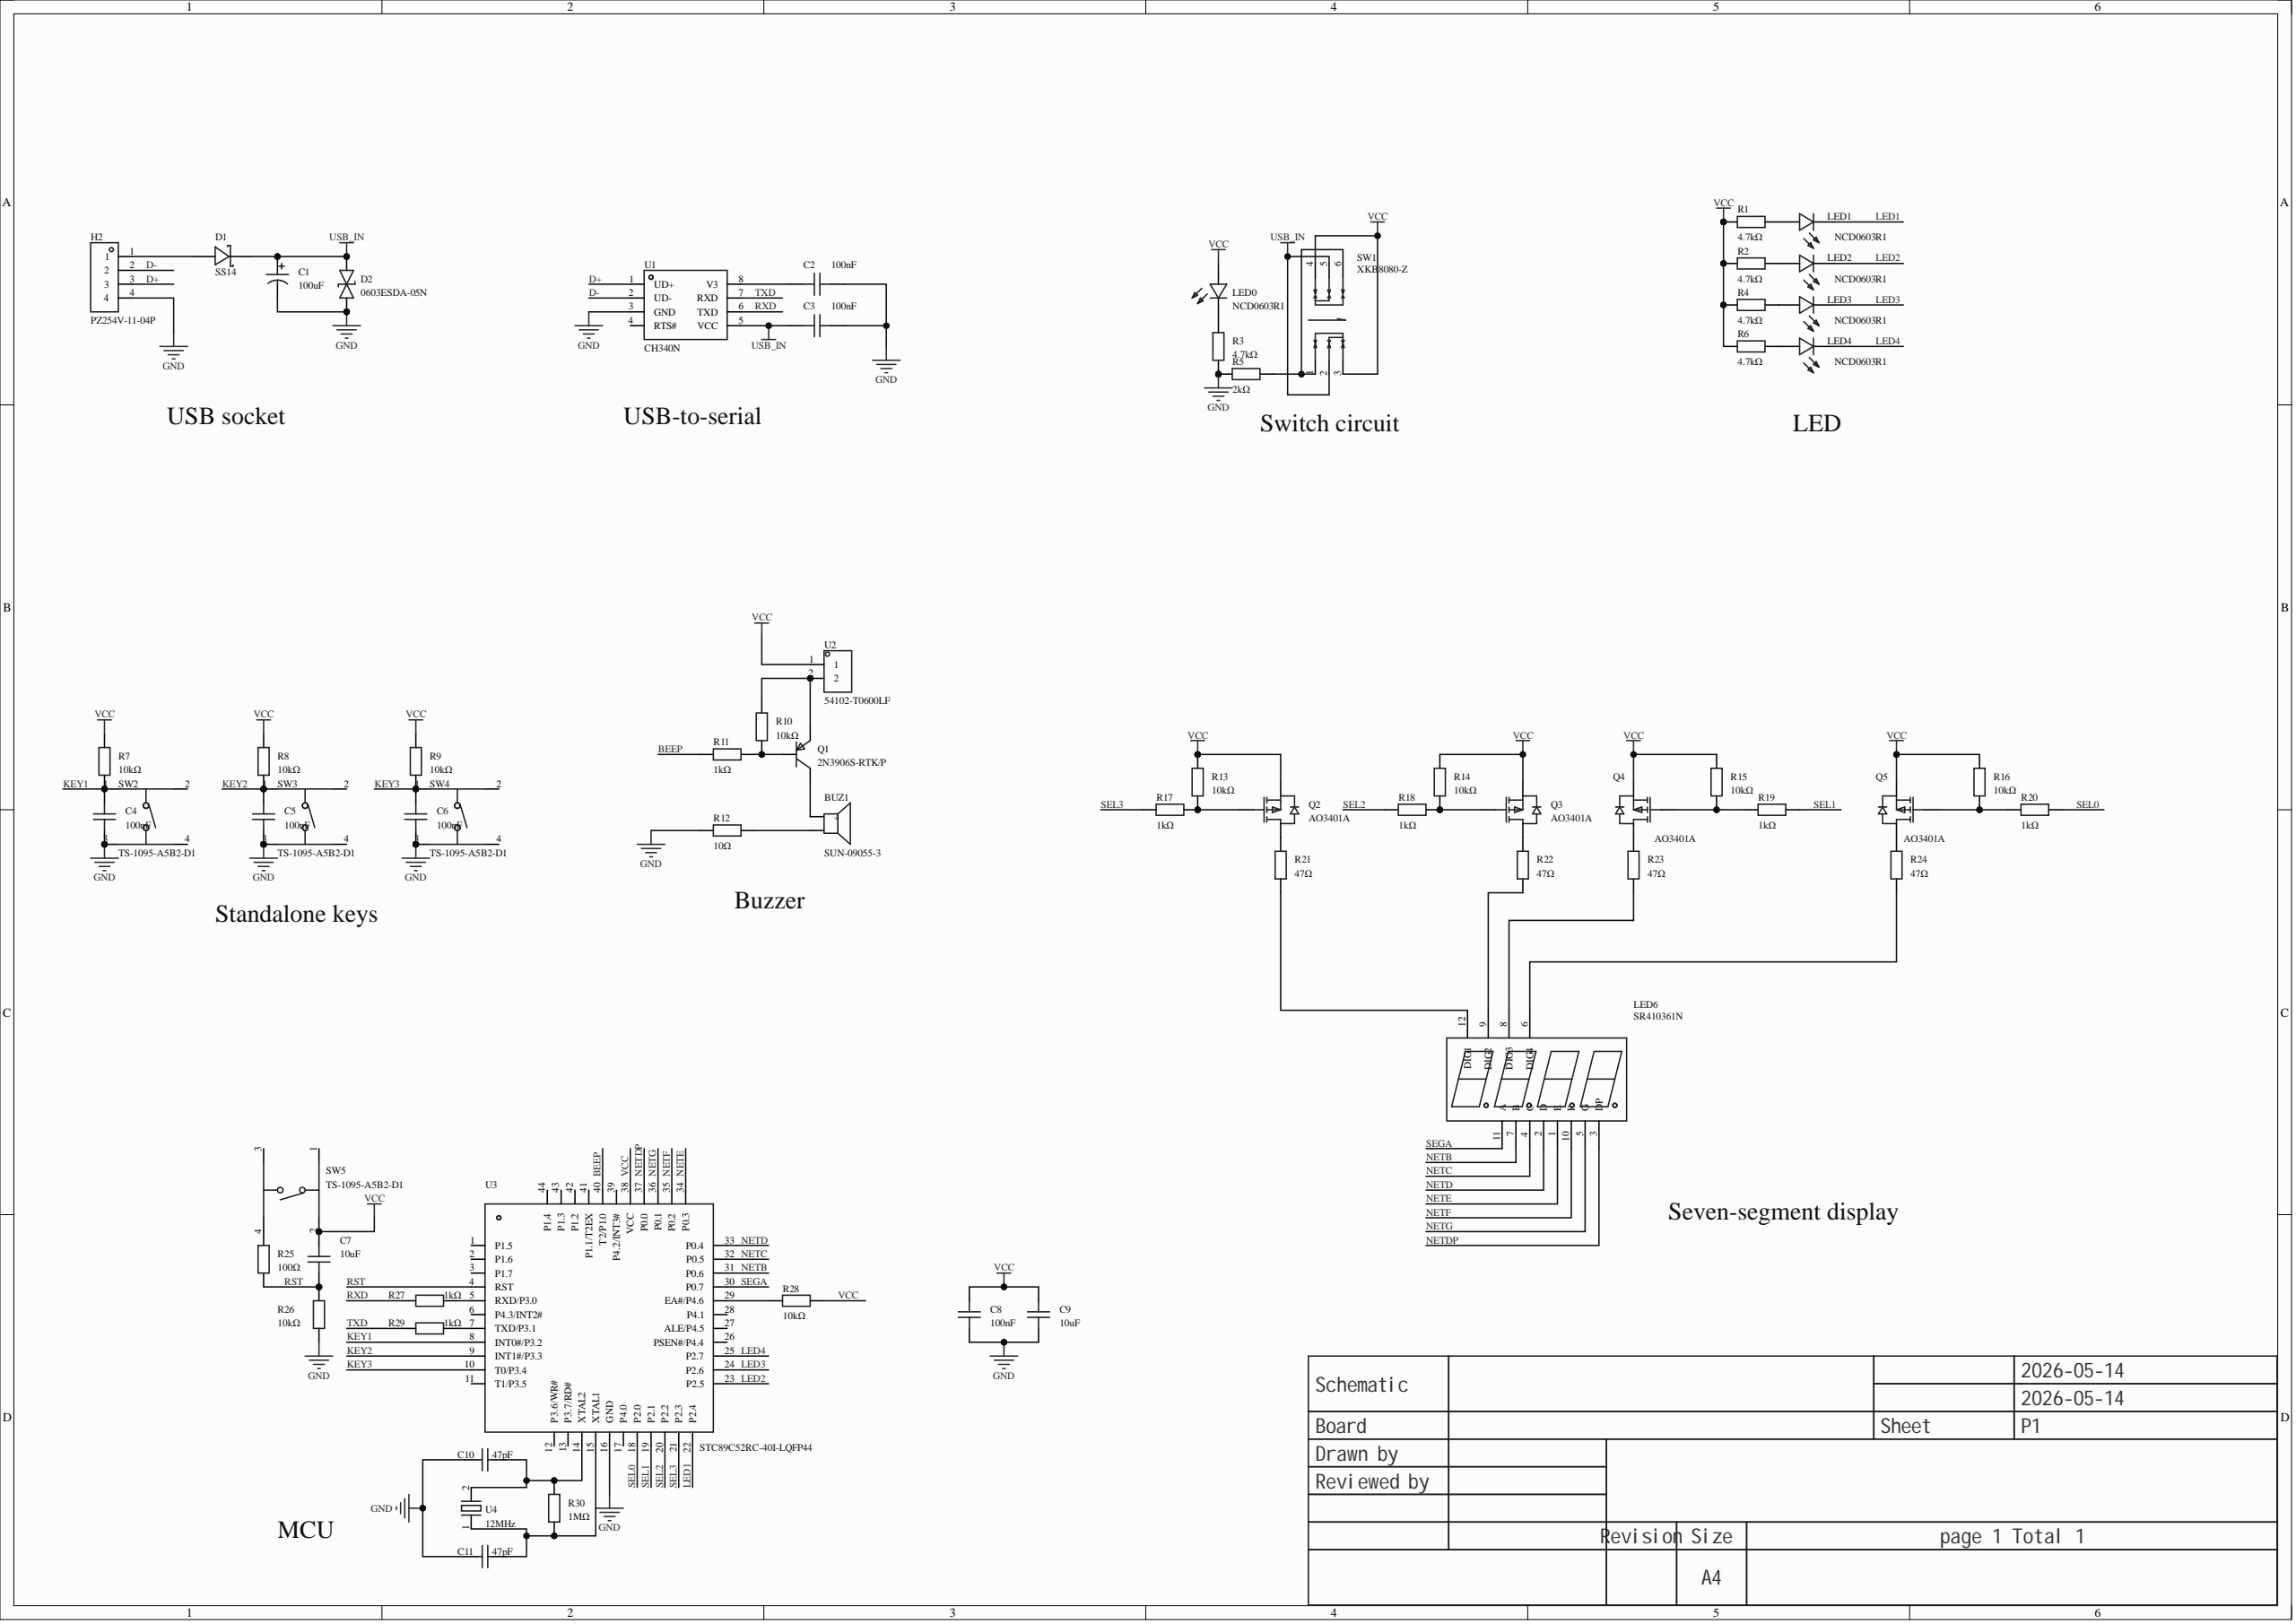Circuit board | Altium Designer | 65 parts | 58 nets
Bill of materials:
Comment,Description,Designator,Footprint,LibRef,Quantity
"SUN-09055-3","Frequency 2800+300Hz, 1.5-5V voltage drive","BUZ1","BUZ-TH_BD9.0-P5.00-D0.6-FD","SUN-09055-3","1"
"100uF","Capacitance: 100uF; Tolerance: ±20%; Rated voltage: 16V; Ripple current: -; ESR: -;","C1","CAP-TH_BD5.0-P2.00-D0.8-FD","KS107M016D07RR0VH2FP0","1"
"100nF","Capacitance: 100nF; Tolerance: ±10%; Rated voltage: 50V; Temperature coefficient: X7R;","C2, C3, C4, C5, C6, C8","C0603","CL10B104KB8NNNC","6"
"10uF","Capacitance: 10uF; Tolerance: ±20%; Rated voltage: 25V; Temperature coefficient: X5R;","C7, C9","C0603","CL10A106MA8NRNC","2"
"47pF","Capacitance: 47pF; Tolerance: ±5%; Rated voltage: 50V; Temperature coefficient: C0G;","C10, C11","C0603","CL10C470JB8NNNC","2"
"SS14","Diode configuration: Discrete; Forward voltage (Vf): 550mV@1A; DC reverse voltage (Vr): 40V; Rectifier current: 1A;","D1","SMA_L4.2-W2.6-LS5.0-RD_1","SS14_C2480","1"
"0603ESDA-05N","Polarity: Bidirectional; Reverse standoff voltage (Vrwm): 5V; Clamping voltage: 100V;","D2","D0603-BI","0603ESDA-05N","1"
"PZ254V-11-04P","Pin structure: 1x4P; Pitch: 2.54mm; Row pitch: -; Round/square pin: Square pin; Mounting type: Through-hole; Number of rows: Single row; Total pins: 4P; Rated current: 3A; Rated voltage: 250V; Mating pin length: 6mm; Housing height: 2.5mm; Termination pin length: 3mm; Contact material: -; Operating temperature: -40℃~+105℃; Color: Black;","H2","HDR-TH_4P-P2.54-V-M","PZ254V-11-04P","1"
"NCD0603R1","LED package type: -; Emission color: Red; Forward voltage (Vf): 1.6V~2.6V; Power: 65mW; Forward current: 25mA; Wavelength: 615nm~630nm; Diode configuration: Discrete diode; Lens color: -; Color temperature: -; Luminous intensity: 220mcd; Viewing angle: 130°; Packaging: -; Operating temperature: -30℃~+85℃;","LED0, LED1, LED2, LED3, LED4","LED0603-RD_RED","NCD0603R1_C84263","5"
"SR410361N","Digits: 4-digit; Character size (inch): 0.36; LED polarity: Common anode; Emission color: Red; Power dissipation (Pd): 50mW;","LED6","LED-SEG-TH_12P-L30.0-W14.0-P2.54-S10.26-BL","SR410361N","1"
"2N3906S-RTK/P","Transistor type: PNP; Collector current (Ic): 200mA; Collector-emitter breakdown voltage (Vceo): 40V; Power dissipation (Pd): 350mW; DC current gain (hFE): 100@10mA,1V;","Q1","SOT-23-3_L2.9-W1.6-P1.90-LS2.8-TR-CW","2N3906S-RTK/P_C147294","1"
"AO3401A","","Q2, Q3, Q4, Q5","SOT-23_L2.9-W1.3-P1.90-LS2.4-BR","AO3401A_C15127","4"
"4.7kΩ","Resistor type: Thick-film resistor; Resistance: 4.7kΩ; Tolerance: ±1%; Power: 100mW; Operating voltage: 75V; Temperature coefficient: ±100ppm/?;","R1, R2, R3, R4, R6","R0603","RC0603FR-074K7L","5"
"2kΩ","Resistor type: Thick-film resistor; Resistance: 2kΩ; Tolerance: ±1%; Power: 100mW; Operating voltage: 75V; Temperature coefficient: ±100ppm/?;","R5","R0603","0603WAF2001T5E","1"
"10kΩ","Resistor type: Thick-film resistor; Resistance: 10kΩ; Tolerance: ±1%; Power: 100mW; Operating voltage: 75V; Temperature coefficient: ±100ppm/?;","R7, R8, R9, R10, R13, R14, R15, R16, R26, R28","R0603","0603WAF1002T5E","10"
"1kΩ","Resistor type: Thick-film resistor; Resistance: 1kΩ; Tolerance: ±1%; Power: 100mW; Operating voltage: 75V; Temperature coefficient: ±100ppm/?;","R11, R17, R18, R19, R20, R27, R29","R0603","RC0603FR-071KL","7"
"10Ω","Resistor type: Thick-film resistor; Resistance: 10Ω; Tolerance: ±1%; Power: 100mW; Operating voltage: 75V; Temperature coefficient: ±400ppm/?;","R12","R0603","0603WAF100JT5E","1"
"47Ω","Resistor type: Thick-film resistor; Resistance: 47Ω; Tolerance: ±1%; Power: 100mW; Operating voltage: 75V; Temperature coefficient: ±100ppm/?;","R21, R22, R23, R24","R0603","0603WAF470JT5E","4"
"100Ω","Resistor type: Thick-film resistor; Resistance: 100Ω; Tolerance: ±1%; Power: 100mW; Max operating voltage: 75V; Temperature coefficient: ±100ppm/?;","R25","R0603","RC0603FR-07100RL","1"
"1MΩ","Resistor type: Thick-film resistor; Resistance: 1MΩ; Tolerance: ±1%; Power: 100mW; Max operating voltage: 75V; Temperature coefficient: ±100ppm/?;","R30","R0603","0603WAF1004T5E","1"
"XKB8080-Z","Latching/non-latching: Latching; Mounting type: Through-hole; Contact current: 100mA; Rated voltage: 30V; With lamp: Without; Actuating force: 1.6N; Operating life: 10万 cycles;","SW1","SW-TH_6P-L8.0-W8.0-P2.50","XKB8080-Z","1"
"TS-1095-A5B2-D1","Circuit configuration: SPST; Button shape: Round button; Actuating force: 180gf; Mounting type: Through-hole; Switch length: 6mm; Switch width: 6mm; Switch height: 6mm; With bracket: Without; Mechanical life: -;","SW2, SW3, SW4, SW5","SW-TH_4P-L6.0-W6.0-P4.50-LS6.5","TS-1095-A5B2-D1","4"
"CH340N","Function: USB-to-serial; Interface protocol: USB 2.0; Channels: -; Data rate: 2Mbps;","U1","SOP-8_L5.0-W4.0-P1.27-LS6.0-BL","CH340N_C506813","1"
"54102-T0600LF","Pin structure: -; Pitch: 2.54mm; Row pitch: 2.54mm; Round/square pin: Square pin; Mounting type: Through-hole; Number of rows: Double row; Rated current: 3A; Rated voltage: -; Mating pin length: 5.84mm; Housing height: 2.54mm; Termination pin length: 2.79mm; Contact material: Phosphor bronze; Contact plating: Tin; Operating temperature: -65℃~+125℃; Color: Black;","U2","HDR-TH_2P-P2.54-V-M-R2-C1-S2.54","54102-T0600LF","1"
"STC89C52RC-40I-LQFP44","CPU core: 51 family;","U3","LQFP-44_L10.0-W10.0-P0.80-LS12.0-BL","STC89C52RC-40I-LQFP44","1"
"12MHz","Crystal type: Through-hole crystal; Frequency: 12MHz; Frequency tolerance at room temperature: ±20ppm; Load capacitance: 18pF; Frequency stability: ±30ppm;","U4","HC-49S_L11.4-W4.7-P4.88-D0.4","049ST2-12.000F18DTLJL","1"
Netlist (Protel format):
[
BUZ1
BUZ-TH_BD9.0-P5.00-D0.6-FD
SUN-09055-3



]
[
C1
CAP-TH_BD5.0-P2.00-D0.8-FD
100uF



]
[
C2
C0603
100nF



]
[
C3
C0603
100nF



]
[
C4
C0603
100nF



]
[
C5
C0603
100nF



]
[
C6
C0603
100nF



]
[
C7
C0603
10uF



]
[
C8
C0603
100nF



]
[
C9
C0603
10uF



]
[
C10
C0603
47pF



]
[
C11
C0603
47pF



]
[
D1
SMA_L4.2-W2.6-LS5.0-RD_1
SS14



]
[
D2
D0603-BI
0603ESDA-05N



]
[
H2
HDR-TH_4P-P2.54-V-M
PZ254V-11-04P



]
[
LED0
LED0603-RD_RED
NCD0603R1



]
[
LED1
LED0603-RD_RED
NCD0603R1



]
[
LED2
LED0603-RD_RED
NCD0603R1



]
[
LED3
LED0603-RD_RED
NCD0603R1



]
[
LED4
LED0603-RD_RED
NCD0603R1



]
[
LED6
LED-SEG-TH_12P-L30.0-W14.0-P2.54-S10.26-BL
SR410361N



]
[
Q1
SOT-23-3_L2.9-W1.6-P1.90-LS2.8-TR-CW
2N3906S-RTK/P



]
[
Q2
SOT-23_L2.9-W1.3-P1.90-LS2.4-BR
AO3401A



]
[
Q3
SOT-23_L2.9-W1.3-P1.90-LS2.4-BR
AO3401A



]
[
Q4
SOT-23_L2.9-W1.3-P1.90-LS2.4-BR
AO3401A



]
[
Q5
SOT-23_L2.9-W1.3-P1.90-LS2.4-BR
AO3401A



]
[
R1
R0603
4.7kΩ



]
[
R2
R0603
4.7kΩ



]
[
R3
R0603
4.7kΩ



]
[
R4
R0603
4.7kΩ



]
[
R5
R0603
2kΩ



]
[
R6
R0603
4.7kΩ



]
[
R7
R0603
10kΩ



]
[
R8
R0603
10kΩ



]
[
R9
R0603
10kΩ



]
[
R10
R0603
10kΩ



]
[
R11
R0603
1kΩ



]
[
R12
R0603
10Ω



]
[
R13
R0603
10kΩ



]
[
R14
R0603
10kΩ



]
[
R15
R0603
10kΩ



]
[
R16
R0603
10kΩ



]
[
R17
R0603
1kΩ



]
[
R18
R0603
1kΩ



]
[
R19
R0603
1kΩ



]
[
R20
R0603
1kΩ



]
[
R21
R0603
47Ω



]
[
R22
R0603
47Ω



]
[
R23
R0603
47Ω



]
[
R24
R0603
47Ω



]
[
R25
R0603
100Ω



]
[
R26
R0603
10kΩ



]
[
R27
R0603
1kΩ



]
[
R28
R0603
10kΩ



]
[
R29
R0603
1kΩ



]
[
R30
R0603
1MΩ



]
[
SW1
SW-TH_6P-L8.0-W8.0-P2.50
XKB8080-Z



]
[
SW2
SW-TH_4P-L6.0-W6.0-P4.50-LS6.5
TS-1095-A5B2-D1



]
[
SW3
SW-TH_4P-L6.0-W6.0-P4.50-LS6.5
TS-1095-A5B2-D1



]
[
SW4
SW-TH_4P-L6.0-W6.0-P4.50-LS6.5
TS-1095-A5B2-D1



]
[
SW5
SW-TH_4P-L6.0-W6.0-P4.50-LS6.5
TS-1095-A5B2-D1



]
[
U1
SOP-8_L5.0-W4.0-P1.27-LS6.0-BL
CH340N



]
[
U2
HDR-TH_2P-P2.54-V-M-R2-C1-S2.54
54102-T0600LF



]
[
U3
LQFP-44_L10.0-W10.0-P0.80-LS12.0-BL
STC89C52RC-40I-LQFP44



]
[
U4
HC-49S_L11.4-W4.7-P4.88-D0.4
12MHz



]
(
VCC
C7-2
C8-2
C9-2
LED0-2
Q2-2
Q3-2
Q4-2
Q5-2
R1-1
R2-1
R4-1
R6-1
R7-2
R8-2
R9-2
R13-2
R14-2
R15-2
R16-2
R28-2
SW1-3
SW1-4
SW5-2
U2-1
U3-38
)
(
USB_IN
C1-1
C3-1
D1-1
D2-2
SW1-2
SW1-5
U1-5
)
(
TXD
R29-1
U1-7
)
(
SEL3
R17-1
U3-21
)
(
SEL2
R18-1
U3-20
)
(
SEL1
R19-2
U3-19
)
(
SEL0
R20-2
U3-18
)
(
SEGA
LED6-11
U3-30
)
(
RXD
R27-1
U1-6
)
(
RST
C7-1
R25-1
R26-2
U3-4
)
(
NetR29_2
R29-2
U3-7
)
(
NetR28_1
R28-1
U3-29
)
(
NetR27_2
R27-2
U3-5
)
(
NetR25_2
R25-2
SW5-4
)
(
NetR5_2
R5-2
SW1-1
SW1-6
)
(
NetQ5_3
Q5-3
R24-2
)
(
NetQ5_1
Q5-1
R16-1
R20-1
)
(
NetQ4_3
Q4-3
R23-2
)
(
NetQ4_1
Q4-1
R15-1
R19-1
)
(
NetQ3_3
Q3-3
R22-2
)
(
NetQ3_1
Q3-1
R14-1
R18-2
)
(
NetQ2_3
Q2-3
R21-2
)
(
NetQ2_1
Q2-1
R13-1
R17-2
)
(
NetQ1_2
Q1-2
R10-1
R11-2
)
(
NetQ1_1
Q1-1
R10-2
U2-2
)
(
NetLED6_12
LED6-12
R21-1
)
(
NetLED6_9
LED6-9
R22-1
)
(
NetLED6_8
LED6-8
R23-1
)
(
NetLED6_6
LED6-6
R24-1
)
(
NetLED4_2
LED4-2
R6-2
)
(
NetLED3_2
LED3-2
R4-2
)
(
NetLED2_2
LED2-2
R2-2
)
(
NetLED1_2
LED1-2
R1-2
)
(
NetLED0_1
LED0-1
R3-2
)
(
NETG
LED6-5
U3-36
)
(
NETF
LED6-10
U3-35
)
(
NETE
LED6-1
U3-34
)
(
NETDP
LED6-3
U3-37
)
(
NetD1_2
D1-2
H2-1
)
(
NETD
LED6-2
U3-33
)
(
NetC11_2
C11-2
R30-1
U3-15
U4-1
)
(
NetC10_2
C10-2
R30-2
U3-14
U4-2
)
(
NetC2_1
C2-1
U1-8
)
(
NETC
LED6-4
U3-32
)
(
NetBUZ1_2
BUZ1-2
R12-2
)
(
NetBUZ1_1
BUZ1-1
Q1-3
)
(
NETB
LED6-7
U3-31
)
(
LED4
LED4-1
U3-25
)
(
LED3
LED3-1
U3-24
)
(
LED2
LED2-1
U3-23
)
(
LED1
LED1-1
U3-22
)
(
KEY3
C6-2
R9-1
SW4-1
U3-10
)
(
KEY2
C5-2
R8-1
SW3-1
U3-9
)
(
KEY1
C4-2
R7-1
SW2-1
U3-8
)
(
GND
C1-2
C2-2
C3-2
C4-1
C5-1
C6-1
C8-1
C9-1
C10-1
C11-1
D2-1
H2-4
R3-1
R5-1
R12-1
R26-1
SW2-3
SW3-3
SW4-3
U1-3
U3-16
)
(
D-
H2-2
U1-2
)
(
D+
H2-3
U1-1
)
(
BEEP
R11-1
U3-40
)